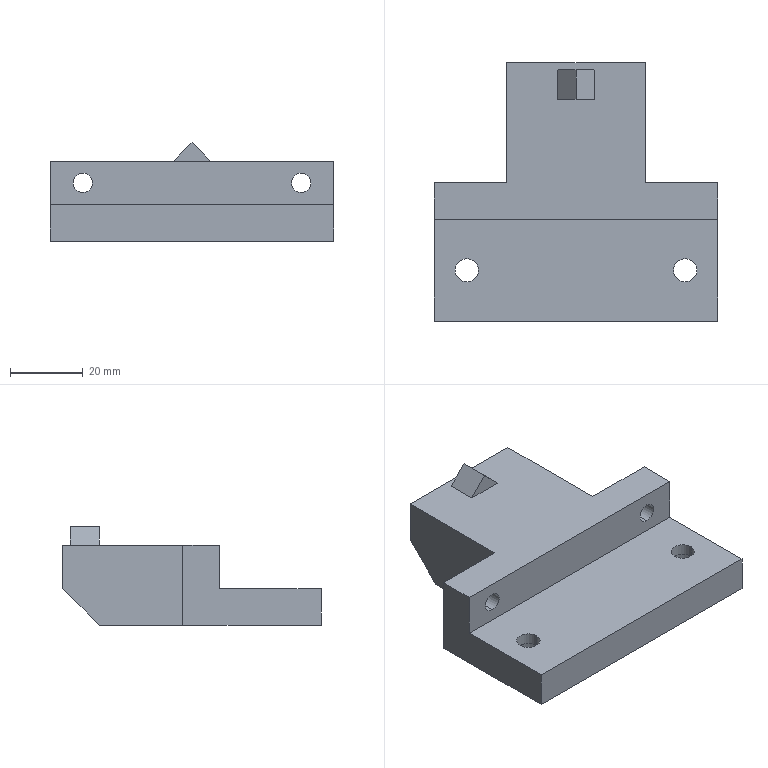Part | STEP file | Correction clamp plate_default<machined> | 1 solid | 37 faces | box 78 x 71 x 27 mm | volume 62305 mm3 | plane 21 | cylinder 16 | commonest cylinder face diameters 5.3 x4 6.4 x4 10 x4 11 x4